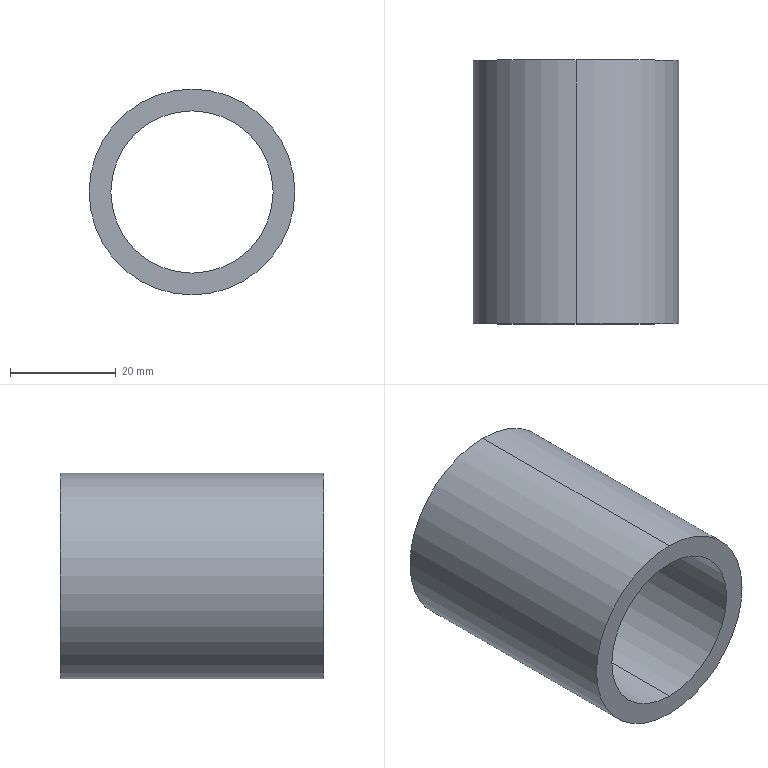Part | SolidWorks | features 3DProfileFeature 1, Extrusion 1, HoleWzd 1 | 1 solid | 6 faces | box 39 x 50 x 39 mm | volume 22597 mm3 | cylinder 4 | plane 2 | commonest cylinder face diameters 30.75 x2 39 x2
STEP:
#1=CARTESIAN_POINT('',(0.,0.,-15.375));
#2=VERTEX_POINT('',#1);
#3=CARTESIAN_POINT('',(0.,0.,15.375));
#4=VERTEX_POINT('',#3);
#5=CARTESIAN_POINT('',(0.,0.,0.));
#6=DIRECTION('',(0.,1.,0.));
#7=DIRECTION('',(0.,0.,1.));
#8=AXIS2_PLACEMENT_3D('',#5,#6,#7);
#9=CIRCLE('',#8,15.375);
#10=EDGE_CURVE('',#2,#4,#9,.T.);
#11=ORIENTED_EDGE('',*,*,#10,.F.);
#12=CARTESIAN_POINT('',(0.,50.,-15.375));
#13=VERTEX_POINT('',#12);
#14=CARTESIAN_POINT('',(0.,50.,-15.375));
#15=DIRECTION('',(0.,1.,0.));
#16=VECTOR('',#15,1000.);
#17=LINE('',#14,#16);
#18=EDGE_CURVE('',#2,#13,#17,.T.);
#19=ORIENTED_EDGE('',*,*,#18,.T.);
#20=CARTESIAN_POINT('',(0.,50.,15.375));
#21=VERTEX_POINT('',#20);
#22=CARTESIAN_POINT('',(0.,50.,0.));
#23=DIRECTION('',(0.,1.,0.));
#24=DIRECTION('',(0.,0.,1.));
#25=AXIS2_PLACEMENT_3D('',#22,#23,#24);
#26=CIRCLE('',#25,15.375);
#27=EDGE_CURVE('',#13,#21,#26,.T.);
#28=ORIENTED_EDGE('',*,*,#27,.T.);
#29=CARTESIAN_POINT('',(0.,50.,15.375));
#30=DIRECTION('',(0.,1.,0.));
#31=VECTOR('',#30,1000.);
#32=LINE('',#29,#31);
#33=EDGE_CURVE('',#4,#21,#32,.T.);
#34=ORIENTED_EDGE('',*,*,#33,.F.);
#35=EDGE_LOOP('',(#11,#19,#28,#34));
#36=FACE_OUTER_BOUND('',#35,.T.);
#37=CARTESIAN_POINT('',(0.,50.,0.));
#38=DIRECTION('',(0.,1.,0.));
#39=DIRECTION('',(0.,0.,1.));
#40=AXIS2_PLACEMENT_3D('',#37,#38,#39);
#41=CYLINDRICAL_SURFACE('',#40,15.375);
#42=ADVANCED_FACE('',(#36),#41,.F.);
#43=CARTESIAN_POINT('',(0.,50.,19.5));
#44=VERTEX_POINT('',#43);
#45=CARTESIAN_POINT('',(0.,50.,-19.5));
#46=VERTEX_POINT('',#45);
#47=CARTESIAN_POINT('',(0.,50.,0.));
#48=DIRECTION('',(0.,1.,0.));
#49=DIRECTION('',(0.,0.,1.));
#50=AXIS2_PLACEMENT_3D('',#47,#48,#49);
#51=CIRCLE('',#50,19.5);
#52=EDGE_CURVE('',#44,#46,#51,.T.);
#53=ORIENTED_EDGE('',*,*,#52,.F.);
#54=CARTESIAN_POINT('',(0.,0.,19.5));
#55=VERTEX_POINT('',#54);
#56=CARTESIAN_POINT('',(0.,50.,19.5));
#57=DIRECTION('',(0.,-1.,0.));
#58=VECTOR('',#57,1000.);
#59=LINE('',#56,#58);
#60=EDGE_CURVE('',#44,#55,#59,.T.);
#61=ORIENTED_EDGE('',*,*,#60,.T.);
#62=CARTESIAN_POINT('',(0.,0.,-19.5));
#63=VERTEX_POINT('',#62);
#64=CARTESIAN_POINT('',(0.,0.,0.));
#65=DIRECTION('',(0.,1.,0.));
#66=DIRECTION('',(0.,0.,1.));
#67=AXIS2_PLACEMENT_3D('',#64,#65,#66);
#68=CIRCLE('',#67,19.5);
#69=EDGE_CURVE('',#55,#63,#68,.T.);
#70=ORIENTED_EDGE('',*,*,#69,.T.);
#71=CARTESIAN_POINT('',(0.,50.,-19.5));
#72=DIRECTION('',(0.,-1.,0.));
#73=VECTOR('',#72,1000.);
#74=LINE('',#71,#73);
#75=EDGE_CURVE('',#46,#63,#74,.T.);
#76=ORIENTED_EDGE('',*,*,#75,.F.);
#77=EDGE_LOOP('',(#53,#61,#70,#76));
#78=FACE_OUTER_BOUND('',#77,.T.);
#79=CARTESIAN_POINT('',(0.,50.,0.));
#80=DIRECTION('',(0.,-1.,0.));
#81=DIRECTION('',(0.,0.,-1.));
#82=AXIS2_PLACEMENT_3D('',#79,#80,#81);
#83=CYLINDRICAL_SURFACE('',#82,19.5);
#84=ADVANCED_FACE('',(#78),#83,.T.);
#85=ORIENTED_EDGE('',*,*,#60,.F.);
#86=CARTESIAN_POINT('',(0.,50.,0.));
#87=DIRECTION('',(0.,1.,0.));
#88=DIRECTION('',(0.,0.,1.));
#89=AXIS2_PLACEMENT_3D('',#86,#87,#88);
#90=CIRCLE('',#89,19.5);
#91=EDGE_CURVE('',#46,#44,#90,.T.);
#92=ORIENTED_EDGE('',*,*,#91,.F.);
#93=ORIENTED_EDGE('',*,*,#75,.T.);
#94=CARTESIAN_POINT('',(0.,0.,0.));
#95=DIRECTION('',(0.,1.,0.));
#96=DIRECTION('',(0.,0.,1.));
#97=AXIS2_PLACEMENT_3D('',#94,#95,#96);
#98=CIRCLE('',#97,19.5);
#99=EDGE_CURVE('',#63,#55,#98,.T.);
#100=ORIENTED_EDGE('',*,*,#99,.T.);
#101=EDGE_LOOP('',(#85,#92,#93,#100));
#102=FACE_OUTER_BOUND('',#101,.T.);
#103=CARTESIAN_POINT('',(0.,50.,0.));
#104=DIRECTION('',(0.,-1.,0.));
#105=DIRECTION('',(0.,0.,-1.));
#106=AXIS2_PLACEMENT_3D('',#103,#104,#105);
#107=CYLINDRICAL_SURFACE('',#106,19.5);
#108=ADVANCED_FACE('',(#102),#107,.T.);
#109=CARTESIAN_POINT('',(0.,50.,0.));
#110=DIRECTION('',(0.,1.,0.));
#111=DIRECTION('',(0.,0.,1.));
#112=AXIS2_PLACEMENT_3D('',#109,#110,#111);
#113=CIRCLE('',#112,15.375);
#114=EDGE_CURVE('',#21,#13,#113,.T.);
#115=ORIENTED_EDGE('',*,*,#114,.F.);
#116=ORIENTED_EDGE('',*,*,#27,.F.);
#117=EDGE_LOOP('',(#115,#116));
#118=FACE_BOUND('',#117,.T.);
#119=ORIENTED_EDGE('',*,*,#91,.T.);
#120=ORIENTED_EDGE('',*,*,#52,.T.);
#121=EDGE_LOOP('',(#119,#120));
#122=FACE_OUTER_BOUND('',#121,.T.);
#123=CARTESIAN_POINT('',(0.,50.,0.));
#124=DIRECTION('',(0.,1.,0.));
#125=DIRECTION('',(0.,0.,1.));
#126=AXIS2_PLACEMENT_3D('',#123,#124,#125);
#127=PLANE('',#126);
#128=ADVANCED_FACE('',(#118,#122),#127,.T.);
#129=CARTESIAN_POINT('',(0.,0.,0.));
#130=DIRECTION('',(0.,1.,0.));
#131=DIRECTION('',(0.,0.,1.));
#132=AXIS2_PLACEMENT_3D('',#129,#130,#131);
#133=CIRCLE('',#132,15.375);
#134=EDGE_CURVE('',#4,#2,#133,.T.);
#135=ORIENTED_EDGE('',*,*,#134,.T.);
#136=ORIENTED_EDGE('',*,*,#10,.T.);
#137=EDGE_LOOP('',(#135,#136));
#138=FACE_BOUND('',#137,.T.);
#139=ORIENTED_EDGE('',*,*,#99,.F.);
#140=ORIENTED_EDGE('',*,*,#69,.F.);
#141=EDGE_LOOP('',(#139,#140));
#142=FACE_OUTER_BOUND('',#141,.T.);
#143=CARTESIAN_POINT('',(0.,0.,0.));
#144=DIRECTION('',(0.,1.,0.));
#145=DIRECTION('',(0.,0.,1.));
#146=AXIS2_PLACEMENT_3D('',#143,#144,#145);
#147=PLANE('',#146);
#148=ADVANCED_FACE('',(#138,#142),#147,.F.);
#149=ORIENTED_EDGE('',*,*,#18,.F.);
#150=ORIENTED_EDGE('',*,*,#134,.F.);
#151=ORIENTED_EDGE('',*,*,#33,.T.);
#152=ORIENTED_EDGE('',*,*,#114,.T.);
#153=EDGE_LOOP('',(#149,#150,#151,#152));
#154=FACE_OUTER_BOUND('',#153,.T.);
#155=CARTESIAN_POINT('',(0.,50.,0.));
#156=DIRECTION('',(0.,1.,0.));
#157=DIRECTION('',(0.,0.,1.));
#158=AXIS2_PLACEMENT_3D('',#155,#156,#157);
#159=CYLINDRICAL_SURFACE('',#158,15.375);
#160=ADVANCED_FACE('',(#154),#159,.F.);
#161=CLOSED_SHELL('',(#42,#84,#108,#128,#148,#160));
#162=MANIFOLD_SOLID_BREP('',#161);
#163=CARTESIAN_POINT('',(0.,0.,0.));
#164=DIRECTION('',(0.,0.,1.));
#165=DIRECTION('',(1.,0.,0.));
#166=AXIS2_PLACEMENT_3D('',#163,#164,#165);
#167=(LENGTH_UNIT()NAMED_UNIT(*)SI_UNIT(.MILLI.,.METRE.));
#168=UNCERTAINTY_MEASURE_WITH_UNIT(LENGTH_MEASURE(0.00001),#167,'','');
#169=(NAMED_UNIT(*)PLANE_ANGLE_UNIT()SI_UNIT($,.RADIAN.));
#170=(NAMED_UNIT(*)SI_UNIT($,.STERADIAN.)SOLID_ANGLE_UNIT());
#171=(GEOMETRIC_REPRESENTATION_CONTEXT(3)GLOBAL_UNCERTAINTY_ASSIGNED_CONTEXT((#168))GLOBAL_UNIT_ASSIGNED_CONTEXT((#167,#169,#170))REPRESENTATION_CONTEXT('',''));
#172=ADVANCED_BREP_SHAPE_REPRESENTATION('',(#162,#166),#171);